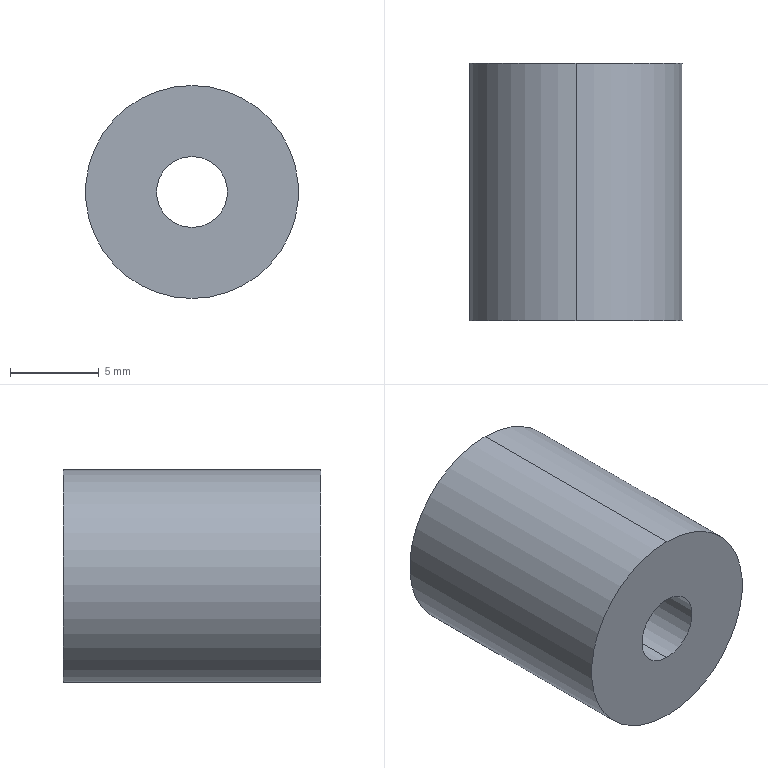Part | STEP file | polyurethane anti-collision post | 1 solid | 9 faces | box 12 x 14.5 x 12 mm | volume 1232 mm3 | cylinder 6 | plane 3 | commonest cylinder face diameters 4 x2 8 x2 12 x2
STEP:
#1=CARTESIAN_POINT('',(0.,0.,0.));
#2=DIRECTION('',(0.,0.,1.));
#3=DIRECTION('',(1.,0.,0.));
#4=AXIS2_PLACEMENT_3D('',#1,#2,#3);
#5=CARTESIAN_POINT('',(0.,8.5,4.));
#6=VERTEX_POINT('',#5);
#7=CARTESIAN_POINT('',(0.,14.5,4.));
#8=VERTEX_POINT('',#7);
#9=CARTESIAN_POINT('',(0.,14.5,4.));
#10=DIRECTION('',(0.,1.,0.));
#11=VECTOR('',#10,1.);
#12=LINE('',#9,#11);
#13=CARTESIAN_POINT('',(0.,14.5,0.));
#14=DIRECTION('',(0.,1.,0.));
#15=DIRECTION('',(0.,0.,1.));
#16=AXIS2_PLACEMENT_3D('',#13,#14,#15);
#17=CYLINDRICAL_SURFACE('',#16,4.);
#18=CARTESIAN_POINT('',(6.283,0.));
#19=DIRECTION('',(0.,1.));
#20=VECTOR('',#19,1.);
#21=LINE('',#18,#20);
#22=(GEOMETRIC_REPRESENTATION_CONTEXT(2)PARAMETRIC_REPRESENTATION_CONTEXT()REPRESENTATION_CONTEXT('',''));
#23=DEFINITIONAL_REPRESENTATION('',(#21),#22);
#24=PCURVE('',#17,#23);
#25=CARTESIAN_POINT('',(0.,14.5,0.));
#26=DIRECTION('',(0.,1.,0.));
#27=DIRECTION('',(0.,0.,1.));
#28=AXIS2_PLACEMENT_3D('',#25,#26,#27);
#29=CYLINDRICAL_SURFACE('',#28,4.);
#30=CARTESIAN_POINT('',(0.,0.));
#31=DIRECTION('',(0.,1.));
#32=VECTOR('',#31,1.);
#33=LINE('',#30,#32);
#34=(GEOMETRIC_REPRESENTATION_CONTEXT(2)PARAMETRIC_REPRESENTATION_CONTEXT()REPRESENTATION_CONTEXT('',''));
#35=DEFINITIONAL_REPRESENTATION('',(#33),#34);
#36=PCURVE('',#29,#35);
#37=SURFACE_CURVE('',#12,(#24,#36),.PCURVE_S1.);
#38=EDGE_CURVE('',#6,#8,#37,.T.);
#39=ORIENTED_EDGE('',*,*,#38,.T.);
#40=CARTESIAN_POINT('',(0.,14.5,-4.));
#41=VERTEX_POINT('',#40);
#42=CARTESIAN_POINT('',(0.,14.5,0.));
#43=DIRECTION('',(0.,1.,0.));
#44=DIRECTION('',(0.,0.,1.));
#45=AXIS2_PLACEMENT_3D('',#42,#43,#44);
#46=CIRCLE('',#45,4.);
#47=CARTESIAN_POINT('',(0.,0.));
#48=DIRECTION('',(1.,0.));
#49=VECTOR('',#48,1.);
#50=LINE('',#47,#49);
#51=(GEOMETRIC_REPRESENTATION_CONTEXT(2)PARAMETRIC_REPRESENTATION_CONTEXT()REPRESENTATION_CONTEXT('',''));
#52=DEFINITIONAL_REPRESENTATION('',(#50),#51);
#53=PCURVE('',#17,#52);
#54=CARTESIAN_POINT('',(0.,14.5,0.));
#55=DIRECTION('',(0.,1.,0.));
#56=DIRECTION('',(0.,0.,1.));
#57=AXIS2_PLACEMENT_3D('',#54,#55,#56);
#58=PLANE('',#57);
#59=CARTESIAN_POINT('',(0.,0.));
#60=DIRECTION('',(1.,0.));
#61=AXIS2_PLACEMENT_2D('',#59,#60);
#62=CIRCLE('',#61,4.);
#63=(GEOMETRIC_REPRESENTATION_CONTEXT(2)PARAMETRIC_REPRESENTATION_CONTEXT()REPRESENTATION_CONTEXT('',''));
#64=DEFINITIONAL_REPRESENTATION('',(#62),#63);
#65=PCURVE('',#58,#64);
#66=SURFACE_CURVE('',#46,(#53,#65),.PCURVE_S1.);
#67=EDGE_CURVE('',#41,#8,#66,.T.);
#68=ORIENTED_EDGE('',*,*,#67,.F.);
#69=CARTESIAN_POINT('',(0.,8.5,-4.));
#70=VERTEX_POINT('',#69);
#71=CARTESIAN_POINT('',(0.,14.5,-4.));
#72=DIRECTION('',(0.,1.,0.));
#73=VECTOR('',#72,1.);
#74=LINE('',#71,#73);
#75=CARTESIAN_POINT('',(3.142,0.));
#76=DIRECTION('',(0.,1.));
#77=VECTOR('',#76,1.);
#78=LINE('',#75,#77);
#79=(GEOMETRIC_REPRESENTATION_CONTEXT(2)PARAMETRIC_REPRESENTATION_CONTEXT()REPRESENTATION_CONTEXT('',''));
#80=DEFINITIONAL_REPRESENTATION('',(#78),#79);
#81=PCURVE('',#17,#80);
#82=CARTESIAN_POINT('',(3.142,0.));
#83=DIRECTION('',(0.,1.));
#84=VECTOR('',#83,1.);
#85=LINE('',#82,#84);
#86=(GEOMETRIC_REPRESENTATION_CONTEXT(2)PARAMETRIC_REPRESENTATION_CONTEXT()REPRESENTATION_CONTEXT('',''));
#87=DEFINITIONAL_REPRESENTATION('',(#85),#86);
#88=PCURVE('',#29,#87);
#89=SURFACE_CURVE('',#74,(#81,#88),.PCURVE_S1.);
#90=EDGE_CURVE('',#70,#41,#89,.T.);
#91=ORIENTED_EDGE('',*,*,#90,.F.);
#92=CARTESIAN_POINT('',(0.,8.5,0.));
#93=DIRECTION('',(0.,1.,0.));
#94=DIRECTION('',(0.,0.,1.));
#95=AXIS2_PLACEMENT_3D('',#92,#93,#94);
#96=CIRCLE('',#95,4.);
#97=CARTESIAN_POINT('',(0.,-6.));
#98=DIRECTION('',(1.,0.));
#99=VECTOR('',#98,1.);
#100=LINE('',#97,#99);
#101=(GEOMETRIC_REPRESENTATION_CONTEXT(2)PARAMETRIC_REPRESENTATION_CONTEXT()REPRESENTATION_CONTEXT('',''));
#102=DEFINITIONAL_REPRESENTATION('',(#100),#101);
#103=PCURVE('',#17,#102);
#104=CARTESIAN_POINT('',(2.,8.5,0.));
#105=DIRECTION('',(0.,-1.,0.));
#106=DIRECTION('',(0.,0.,-1.));
#107=AXIS2_PLACEMENT_3D('',#104,#105,#106);
#108=PLANE('',#107);
#109=CARTESIAN_POINT('',(-4.,-2.));
#110=CARTESIAN_POINT('',(-4.,4.928));
#111=CARTESIAN_POINT('',(2.,1.464));
#112=CARTESIAN_POINT('',(8.,-2.));
#113=CARTESIAN_POINT('',(2.,-5.464));
#114=CARTESIAN_POINT('',(-4.,-8.928));
#115=CARTESIAN_POINT('',(-4.,-2.));
#116=(BOUNDED_CURVE()B_SPLINE_CURVE(2,(#109,#110,#111,#112,#113,#114,#115),.UNSPECIFIED.,.T.,.F.)B_SPLINE_CURVE_WITH_KNOTS((1,2,2,2,2,1),(-2.094,0.,2.094,4.189,6.283,8.378),.UNSPECIFIED.)CURVE()GEOMETRIC_REPRESENTATION_ITEM()RATIONAL_B_SPLINE_CURVE((1.,0.5,1.,0.5,1.,0.5,1.))REPRESENTATION_ITEM(''));
#117=(GEOMETRIC_REPRESENTATION_CONTEXT(2)PARAMETRIC_REPRESENTATION_CONTEXT()REPRESENTATION_CONTEXT('',''));
#118=DEFINITIONAL_REPRESENTATION('',(#116),#117);
#119=PCURVE('',#108,#118);
#120=SURFACE_CURVE('',#96,(#103,#119),.PCURVE_S1.);
#121=EDGE_CURVE('',#70,#6,#120,.T.);
#122=ORIENTED_EDGE('',*,*,#121,.T.);
#123=EDGE_LOOP('',(#39,#68,#91,#122));
#124=FACE_BOUND('',#123,.F.);
#125=ADVANCED_FACE('',(#124),#17,.F.);
#126=CARTESIAN_POINT('',(0.,0.,2.));
#127=VERTEX_POINT('',#126);
#128=CARTESIAN_POINT('',(0.,8.5,2.));
#129=VERTEX_POINT('',#128);
#130=CARTESIAN_POINT('',(0.,14.5,2.));
#131=DIRECTION('',(0.,1.,0.));
#132=VECTOR('',#131,1.);
#133=LINE('',#130,#132);
#134=CARTESIAN_POINT('',(0.,14.5,0.));
#135=DIRECTION('',(0.,1.,0.));
#136=DIRECTION('',(0.,0.,1.));
#137=AXIS2_PLACEMENT_3D('',#134,#135,#136);
#138=CYLINDRICAL_SURFACE('',#137,2.);
#139=CARTESIAN_POINT('',(6.283,0.));
#140=DIRECTION('',(0.,1.));
#141=VECTOR('',#140,1.);
#142=LINE('',#139,#141);
#143=(GEOMETRIC_REPRESENTATION_CONTEXT(2)PARAMETRIC_REPRESENTATION_CONTEXT()REPRESENTATION_CONTEXT('',''));
#144=DEFINITIONAL_REPRESENTATION('',(#142),#143);
#145=PCURVE('',#138,#144);
#146=CARTESIAN_POINT('',(0.,14.5,0.));
#147=DIRECTION('',(0.,1.,0.));
#148=DIRECTION('',(0.,0.,1.));
#149=AXIS2_PLACEMENT_3D('',#146,#147,#148);
#150=CYLINDRICAL_SURFACE('',#149,2.);
#151=CARTESIAN_POINT('',(0.,0.));
#152=DIRECTION('',(0.,1.));
#153=VECTOR('',#152,1.);
#154=LINE('',#151,#153);
#155=(GEOMETRIC_REPRESENTATION_CONTEXT(2)PARAMETRIC_REPRESENTATION_CONTEXT()REPRESENTATION_CONTEXT('',''));
#156=DEFINITIONAL_REPRESENTATION('',(#154),#155);
#157=PCURVE('',#150,#156);
#158=SURFACE_CURVE('',#133,(#145,#157),.PCURVE_S1.);
#159=EDGE_CURVE('',#127,#129,#158,.T.);
#160=ORIENTED_EDGE('',*,*,#159,.T.);
#161=CARTESIAN_POINT('',(0.,8.5,-2.));
#162=VERTEX_POINT('',#161);
#163=CARTESIAN_POINT('',(0.,8.5,0.));
#164=DIRECTION('',(0.,1.,0.));
#165=DIRECTION('',(0.,0.,1.));
#166=AXIS2_PLACEMENT_3D('',#163,#164,#165);
#167=CIRCLE('',#166,2.);
#168=CARTESIAN_POINT('',(0.,-6.));
#169=DIRECTION('',(1.,0.));
#170=VECTOR('',#169,1.);
#171=LINE('',#168,#170);
#172=(GEOMETRIC_REPRESENTATION_CONTEXT(2)PARAMETRIC_REPRESENTATION_CONTEXT()REPRESENTATION_CONTEXT('',''));
#173=DEFINITIONAL_REPRESENTATION('',(#171),#172);
#174=PCURVE('',#138,#173);
#175=CARTESIAN_POINT('',(-2.,-2.));
#176=CARTESIAN_POINT('',(-2.,1.464));
#177=CARTESIAN_POINT('',(1.,-0.2679));
#178=CARTESIAN_POINT('',(4.,-2.));
#179=CARTESIAN_POINT('',(1.,-3.732));
#180=CARTESIAN_POINT('',(-2.,-5.464));
#181=CARTESIAN_POINT('',(-2.,-2.));
#182=(BOUNDED_CURVE()B_SPLINE_CURVE(2,(#175,#176,#177,#178,#179,#180,#181),.UNSPECIFIED.,.T.,.F.)B_SPLINE_CURVE_WITH_KNOTS((1,2,2,2,2,1),(-2.094,0.,2.094,4.189,6.283,8.378),.UNSPECIFIED.)CURVE()GEOMETRIC_REPRESENTATION_ITEM()RATIONAL_B_SPLINE_CURVE((1.,0.5,1.,0.5,1.,0.5,1.))REPRESENTATION_ITEM(''));
#183=(GEOMETRIC_REPRESENTATION_CONTEXT(2)PARAMETRIC_REPRESENTATION_CONTEXT()REPRESENTATION_CONTEXT('',''));
#184=DEFINITIONAL_REPRESENTATION('',(#182),#183);
#185=PCURVE('',#108,#184);
#186=SURFACE_CURVE('',#167,(#174,#185),.PCURVE_S1.);
#187=EDGE_CURVE('',#162,#129,#186,.T.);
#188=ORIENTED_EDGE('',*,*,#187,.F.);
#189=CARTESIAN_POINT('',(0.,0.,-2.));
#190=VERTEX_POINT('',#189);
#191=CARTESIAN_POINT('',(0.,14.5,-2.));
#192=DIRECTION('',(0.,1.,0.));
#193=VECTOR('',#192,1.);
#194=LINE('',#191,#193);
#195=CARTESIAN_POINT('',(3.142,0.));
#196=DIRECTION('',(0.,1.));
#197=VECTOR('',#196,1.);
#198=LINE('',#195,#197);
#199=(GEOMETRIC_REPRESENTATION_CONTEXT(2)PARAMETRIC_REPRESENTATION_CONTEXT()REPRESENTATION_CONTEXT('',''));
#200=DEFINITIONAL_REPRESENTATION('',(#198),#199);
#201=PCURVE('',#138,#200);
#202=CARTESIAN_POINT('',(3.142,0.));
#203=DIRECTION('',(0.,1.));
#204=VECTOR('',#203,1.);
#205=LINE('',#202,#204);
#206=(GEOMETRIC_REPRESENTATION_CONTEXT(2)PARAMETRIC_REPRESENTATION_CONTEXT()REPRESENTATION_CONTEXT('',''));
#207=DEFINITIONAL_REPRESENTATION('',(#205),#206);
#208=PCURVE('',#150,#207);
#209=SURFACE_CURVE('',#194,(#201,#208),.PCURVE_S1.);
#210=EDGE_CURVE('',#190,#162,#209,.T.);
#211=ORIENTED_EDGE('',*,*,#210,.F.);
#212=CARTESIAN_POINT('',(0.,0.,0.));
#213=DIRECTION('',(0.,1.,0.));
#214=DIRECTION('',(0.,0.,1.));
#215=AXIS2_PLACEMENT_3D('',#212,#213,#214);
#216=CIRCLE('',#215,2.);
#217=CARTESIAN_POINT('',(0.,-14.5));
#218=DIRECTION('',(1.,0.));
#219=VECTOR('',#218,1.);
#220=LINE('',#217,#219);
#221=(GEOMETRIC_REPRESENTATION_CONTEXT(2)PARAMETRIC_REPRESENTATION_CONTEXT()REPRESENTATION_CONTEXT('',''));
#222=DEFINITIONAL_REPRESENTATION('',(#220),#221);
#223=PCURVE('',#138,#222);
#224=CARTESIAN_POINT('',(0.,0.,0.));
#225=DIRECTION('',(0.,1.,0.));
#226=DIRECTION('',(0.,0.,1.));
#227=AXIS2_PLACEMENT_3D('',#224,#225,#226);
#228=PLANE('',#227);
#229=CARTESIAN_POINT('',(0.,0.));
#230=DIRECTION('',(1.,0.));
#231=AXIS2_PLACEMENT_2D('',#229,#230);
#232=CIRCLE('',#231,2.);
#233=(GEOMETRIC_REPRESENTATION_CONTEXT(2)PARAMETRIC_REPRESENTATION_CONTEXT()REPRESENTATION_CONTEXT('',''));
#234=DEFINITIONAL_REPRESENTATION('',(#232),#233);
#235=PCURVE('',#228,#234);
#236=SURFACE_CURVE('',#216,(#223,#235),.PCURVE_S1.);
#237=EDGE_CURVE('',#190,#127,#236,.T.);
#238=ORIENTED_EDGE('',*,*,#237,.T.);
#239=EDGE_LOOP('',(#160,#188,#211,#238));
#240=FACE_BOUND('',#239,.F.);
#241=ADVANCED_FACE('',(#240),#138,.F.);
#242=CARTESIAN_POINT('',(0.,14.5,6.));
#243=VERTEX_POINT('',#242);
#244=CARTESIAN_POINT('',(0.,14.5,-6.));
#245=VERTEX_POINT('',#244);
#246=CARTESIAN_POINT('',(0.,14.5,0.));
#247=DIRECTION('',(0.,1.,0.));
#248=DIRECTION('',(0.,0.,1.));
#249=AXIS2_PLACEMENT_3D('',#246,#247,#248);
#250=CIRCLE('',#249,6.);
#251=CARTESIAN_POINT('',(0.,14.5,0.));
#252=DIRECTION('',(0.,-1.,0.));
#253=DIRECTION('',(0.,0.,-1.));
#254=AXIS2_PLACEMENT_3D('',#251,#252,#253);
#255=CYLINDRICAL_SURFACE('',#254,6.);
#256=CARTESIAN_POINT('',(3.142,0.));
#257=DIRECTION('',(-1.,0.));
#258=VECTOR('',#257,1.);
#259=LINE('',#256,#258);
#260=(GEOMETRIC_REPRESENTATION_CONTEXT(2)PARAMETRIC_REPRESENTATION_CONTEXT()REPRESENTATION_CONTEXT('',''));
#261=DEFINITIONAL_REPRESENTATION('',(#259),#260);
#262=PCURVE('',#255,#261);
#263=CARTESIAN_POINT('',(0.,0.));
#264=DIRECTION('',(1.,0.));
#265=AXIS2_PLACEMENT_2D('',#263,#264);
#266=CIRCLE('',#265,6.);
#267=(GEOMETRIC_REPRESENTATION_CONTEXT(2)PARAMETRIC_REPRESENTATION_CONTEXT()REPRESENTATION_CONTEXT('',''));
#268=DEFINITIONAL_REPRESENTATION('',(#266),#267);
#269=PCURVE('',#58,#268);
#270=SURFACE_CURVE('',#250,(#262,#269),.PCURVE_S1.);
#271=EDGE_CURVE('',#243,#245,#270,.T.);
#272=ORIENTED_EDGE('',*,*,#271,.F.);
#273=CARTESIAN_POINT('',(0.,0.,6.));
#274=VERTEX_POINT('',#273);
#275=CARTESIAN_POINT('',(0.,14.5,6.));
#276=DIRECTION('',(0.,-1.,0.));
#277=VECTOR('',#276,1.);
#278=LINE('',#275,#277);
#279=CARTESIAN_POINT('',(3.142,0.));
#280=DIRECTION('',(0.,1.));
#281=VECTOR('',#280,1.);
#282=LINE('',#279,#281);
#283=(GEOMETRIC_REPRESENTATION_CONTEXT(2)PARAMETRIC_REPRESENTATION_CONTEXT()REPRESENTATION_CONTEXT('',''));
#284=DEFINITIONAL_REPRESENTATION('',(#282),#283);
#285=PCURVE('',#255,#284);
#286=CARTESIAN_POINT('',(0.,14.5,0.));
#287=DIRECTION('',(0.,-1.,0.));
#288=DIRECTION('',(0.,0.,-1.));
#289=AXIS2_PLACEMENT_3D('',#286,#287,#288);
#290=CYLINDRICAL_SURFACE('',#289,6.);
#291=CARTESIAN_POINT('',(3.142,0.));
#292=DIRECTION('',(0.,1.));
#293=VECTOR('',#292,1.);
#294=LINE('',#291,#293);
#295=(GEOMETRIC_REPRESENTATION_CONTEXT(2)PARAMETRIC_REPRESENTATION_CONTEXT()REPRESENTATION_CONTEXT('',''));
#296=DEFINITIONAL_REPRESENTATION('',(#294),#295);
#297=PCURVE('',#290,#296);
#298=SURFACE_CURVE('',#278,(#285,#297),.PCURVE_S1.);
#299=EDGE_CURVE('',#243,#274,#298,.T.);
#300=ORIENTED_EDGE('',*,*,#299,.T.);
#301=CARTESIAN_POINT('',(0.,0.,-6.));
#302=VERTEX_POINT('',#301);
#303=CARTESIAN_POINT('',(0.,0.,0.));
#304=DIRECTION('',(0.,1.,0.));
#305=DIRECTION('',(0.,0.,1.));
#306=AXIS2_PLACEMENT_3D('',#303,#304,#305);
#307=CIRCLE('',#306,6.);
#308=CARTESIAN_POINT('',(3.142,14.5));
#309=DIRECTION('',(-1.,0.));
#310=VECTOR('',#309,1.);
#311=LINE('',#308,#310);
#312=(GEOMETRIC_REPRESENTATION_CONTEXT(2)PARAMETRIC_REPRESENTATION_CONTEXT()REPRESENTATION_CONTEXT('',''));
#313=DEFINITIONAL_REPRESENTATION('',(#311),#312);
#314=PCURVE('',#255,#313);
#315=CARTESIAN_POINT('',(0.,0.));
#316=DIRECTION('',(1.,0.));
#317=AXIS2_PLACEMENT_2D('',#315,#316);
#318=CIRCLE('',#317,6.);
#319=(GEOMETRIC_REPRESENTATION_CONTEXT(2)PARAMETRIC_REPRESENTATION_CONTEXT()REPRESENTATION_CONTEXT('',''));
#320=DEFINITIONAL_REPRESENTATION('',(#318),#319);
#321=PCURVE('',#228,#320);
#322=SURFACE_CURVE('',#307,(#314,#321),.PCURVE_S1.);
#323=EDGE_CURVE('',#274,#302,#322,.T.);
#324=ORIENTED_EDGE('',*,*,#323,.T.);
#325=CARTESIAN_POINT('',(0.,14.5,-6.));
#326=DIRECTION('',(0.,-1.,0.));
#327=VECTOR('',#326,1.);
#328=LINE('',#325,#327);
#329=CARTESIAN_POINT('',(0.,0.));
#330=DIRECTION('',(0.,1.));
#331=VECTOR('',#330,1.);
#332=LINE('',#329,#331);
#333=(GEOMETRIC_REPRESENTATION_CONTEXT(2)PARAMETRIC_REPRESENTATION_CONTEXT()REPRESENTATION_CONTEXT('',''));
#334=DEFINITIONAL_REPRESENTATION('',(#332),#333);
#335=PCURVE('',#255,#334);
#336=CARTESIAN_POINT('',(6.283,0.));
#337=DIRECTION('',(0.,1.));
#338=VECTOR('',#337,1.);
#339=LINE('',#336,#338);
#340=(GEOMETRIC_REPRESENTATION_CONTEXT(2)PARAMETRIC_REPRESENTATION_CONTEXT()REPRESENTATION_CONTEXT('',''));
#341=DEFINITIONAL_REPRESENTATION('',(#339),#340);
#342=PCURVE('',#290,#341);
#343=SURFACE_CURVE('',#328,(#335,#342),.PCURVE_S1.);
#344=EDGE_CURVE('',#245,#302,#343,.T.);
#345=ORIENTED_EDGE('',*,*,#344,.F.);
#346=EDGE_LOOP('',(#272,#300,#324,#345));
#347=FACE_BOUND('',#346,.T.);
#348=ADVANCED_FACE('',(#347),#255,.T.);
#349=ORIENTED_EDGE('',*,*,#299,.F.);
#350=CARTESIAN_POINT('',(0.,14.5,0.));
#351=DIRECTION('',(0.,1.,0.));
#352=DIRECTION('',(0.,0.,1.));
#353=AXIS2_PLACEMENT_3D('',#350,#351,#352);
#354=CIRCLE('',#353,6.);
#355=CARTESIAN_POINT('',(9.425,0.));
#356=DIRECTION('',(-1.,0.));
#357=VECTOR('',#356,1.);
#358=LINE('',#355,#357);
#359=(GEOMETRIC_REPRESENTATION_CONTEXT(2)PARAMETRIC_REPRESENTATION_CONTEXT()REPRESENTATION_CONTEXT('',''));
#360=DEFINITIONAL_REPRESENTATION('',(#358),#359);
#361=PCURVE('',#290,#360);
#362=CARTESIAN_POINT('',(0.,0.));
#363=DIRECTION('',(1.,0.));
#364=AXIS2_PLACEMENT_2D('',#362,#363);
#365=CIRCLE('',#364,6.);
#366=(GEOMETRIC_REPRESENTATION_CONTEXT(2)PARAMETRIC_REPRESENTATION_CONTEXT()REPRESENTATION_CONTEXT('',''));
#367=DEFINITIONAL_REPRESENTATION('',(#365),#366);
#368=PCURVE('',#58,#367);
#369=SURFACE_CURVE('',#354,(#361,#368),.PCURVE_S1.);
#370=EDGE_CURVE('',#245,#243,#369,.T.);
#371=ORIENTED_EDGE('',*,*,#370,.F.);
#372=ORIENTED_EDGE('',*,*,#344,.T.);
#373=CARTESIAN_POINT('',(0.,0.,0.));
#374=DIRECTION('',(0.,1.,0.));
#375=DIRECTION('',(0.,0.,1.));
#376=AXIS2_PLACEMENT_3D('',#373,#374,#375);
#377=CIRCLE('',#376,6.);
#378=CARTESIAN_POINT('',(9.425,14.5));
#379=DIRECTION('',(-1.,0.));
#380=VECTOR('',#379,1.);
#381=LINE('',#378,#380);
#382=(GEOMETRIC_REPRESENTATION_CONTEXT(2)PARAMETRIC_REPRESENTATION_CONTEXT()REPRESENTATION_CONTEXT('',''));
#383=DEFINITIONAL_REPRESENTATION('',(#381),#382);
#384=PCURVE('',#290,#383);
#385=CARTESIAN_POINT('',(0.,0.));
#386=DIRECTION('',(1.,0.));
#387=AXIS2_PLACEMENT_2D('',#385,#386);
#388=CIRCLE('',#387,6.);
#389=(GEOMETRIC_REPRESENTATION_CONTEXT(2)PARAMETRIC_REPRESENTATION_CONTEXT()REPRESENTATION_CONTEXT('',''));
#390=DEFINITIONAL_REPRESENTATION('',(#388),#389);
#391=PCURVE('',#228,#390);
#392=SURFACE_CURVE('',#377,(#384,#391),.PCURVE_S1.);
#393=EDGE_CURVE('',#302,#274,#392,.T.);
#394=ORIENTED_EDGE('',*,*,#393,.T.);
#395=EDGE_LOOP('',(#349,#371,#372,#394));
#396=FACE_BOUND('',#395,.T.);
#397=ADVANCED_FACE('',(#396),#290,.T.);
#398=CARTESIAN_POINT('',(0.,14.5,0.));
#399=DIRECTION('',(0.,1.,0.));
#400=DIRECTION('',(0.,0.,1.));
#401=AXIS2_PLACEMENT_3D('',#398,#399,#400);
#402=CIRCLE('',#401,4.);
#403=CARTESIAN_POINT('',(0.,0.));
#404=DIRECTION('',(1.,0.));
#405=AXIS2_PLACEMENT_2D('',#403,#404);
#406=CIRCLE('',#405,4.);
#407=(GEOMETRIC_REPRESENTATION_CONTEXT(2)PARAMETRIC_REPRESENTATION_CONTEXT()REPRESENTATION_CONTEXT('',''));
#408=DEFINITIONAL_REPRESENTATION('',(#406),#407);
#409=PCURVE('',#58,#408);
#410=CARTESIAN_POINT('',(0.,0.));
#411=DIRECTION('',(1.,0.));
#412=VECTOR('',#411,1.);
#413=LINE('',#410,#412);
#414=(GEOMETRIC_REPRESENTATION_CONTEXT(2)PARAMETRIC_REPRESENTATION_CONTEXT()REPRESENTATION_CONTEXT('',''));
#415=DEFINITIONAL_REPRESENTATION('',(#413),#414);
#416=PCURVE('',#29,#415);
#417=SURFACE_CURVE('',#402,(#409,#416),.PCURVE_S1.);
#418=EDGE_CURVE('',#8,#41,#417,.T.);
#419=ORIENTED_EDGE('',*,*,#418,.F.);
#420=ORIENTED_EDGE('',*,*,#67,.F.);
#421=EDGE_LOOP('',(#419,#420));
#422=FACE_BOUND('',#421,.T.);
#423=ORIENTED_EDGE('',*,*,#370,.T.);
#424=ORIENTED_EDGE('',*,*,#271,.T.);
#425=EDGE_LOOP('',(#423,#424));
#426=FACE_BOUND('',#425,.T.);
#427=ADVANCED_FACE('',(#422,#426),#58,.T.);
#428=CARTESIAN_POINT('',(0.,0.,0.));
#429=DIRECTION('',(0.,1.,0.));
#430=DIRECTION('',(0.,0.,1.));
#431=AXIS2_PLACEMENT_3D('',#428,#429,#430);
#432=CIRCLE('',#431,2.);
#433=CARTESIAN_POINT('',(0.,0.));
#434=DIRECTION('',(1.,0.));
#435=AXIS2_PLACEMENT_2D('',#433,#434);
#436=CIRCLE('',#435,2.);
#437=(GEOMETRIC_REPRESENTATION_CONTEXT(2)PARAMETRIC_REPRESENTATION_CONTEXT()REPRESENTATION_CONTEXT('',''));
#438=DEFINITIONAL_REPRESENTATION('',(#436),#437);
#439=PCURVE('',#228,#438);
#440=CARTESIAN_POINT('',(0.,-14.5));
#441=DIRECTION('',(1.,0.));
#442=VECTOR('',#441,1.);
#443=LINE('',#440,#442);
#444=(GEOMETRIC_REPRESENTATION_CONTEXT(2)PARAMETRIC_REPRESENTATION_CONTEXT()REPRESENTATION_CONTEXT('',''));
#445=DEFINITIONAL_REPRESENTATION('',(#443),#444);
#446=PCURVE('',#150,#445);
#447=SURFACE_CURVE('',#432,(#439,#446),.PCURVE_S1.);
#448=EDGE_CURVE('',#127,#190,#447,.T.);
#449=ORIENTED_EDGE('',*,*,#448,.T.);
#450=ORIENTED_EDGE('',*,*,#237,.T.);
#451=EDGE_LOOP('',(#449,#450));
#452=FACE_BOUND('',#451,.T.);
#453=ORIENTED_EDGE('',*,*,#393,.F.);
#454=ORIENTED_EDGE('',*,*,#323,.F.);
#455=EDGE_LOOP('',(#453,#454));
#456=FACE_BOUND('',#455,.T.);
#457=ADVANCED_FACE('',(#452,#456),#228,.F.);
#458=CARTESIAN_POINT('',(0.,8.5,0.));
#459=DIRECTION('',(0.,1.,0.));
#460=DIRECTION('',(0.,0.,1.));
#461=AXIS2_PLACEMENT_3D('',#458,#459,#460);
#462=CIRCLE('',#461,2.);
#463=CARTESIAN_POINT('',(0.,-6.));
#464=DIRECTION('',(1.,0.));
#465=VECTOR('',#464,1.);
#466=LINE('',#463,#465);
#467=(GEOMETRIC_REPRESENTATION_CONTEXT(2)PARAMETRIC_REPRESENTATION_CONTEXT()REPRESENTATION_CONTEXT('',''));
#468=DEFINITIONAL_REPRESENTATION('',(#466),#467);
#469=PCURVE('',#150,#468);
#470=CARTESIAN_POINT('',(-2.,-2.));
#471=CARTESIAN_POINT('',(-2.,1.464));
#472=CARTESIAN_POINT('',(1.,-0.2679));
#473=CARTESIAN_POINT('',(4.,-2.));
#474=CARTESIAN_POINT('',(1.,-3.732));
#475=CARTESIAN_POINT('',(-2.,-5.464));
#476=CARTESIAN_POINT('',(-2.,-2.));
#477=(BOUNDED_CURVE()B_SPLINE_CURVE(2,(#470,#471,#472,#473,#474,#475,#476),.UNSPECIFIED.,.T.,.F.)B_SPLINE_CURVE_WITH_KNOTS((1,2,2,2,2,1),(-2.094,0.,2.094,4.189,6.283,8.378),.UNSPECIFIED.)CURVE()GEOMETRIC_REPRESENTATION_ITEM()RATIONAL_B_SPLINE_CURVE((1.,0.5,1.,0.5,1.,0.5,1.))REPRESENTATION_ITEM(''));
#478=(GEOMETRIC_REPRESENTATION_CONTEXT(2)PARAMETRIC_REPRESENTATION_CONTEXT()REPRESENTATION_CONTEXT('',''));
#479=DEFINITIONAL_REPRESENTATION('',(#477),#478);
#480=PCURVE('',#108,#479);
#481=SURFACE_CURVE('',#462,(#469,#480),.PCURVE_S1.);
#482=EDGE_CURVE('',#129,#162,#481,.T.);
#483=ORIENTED_EDGE('',*,*,#482,.F.);
#484=ORIENTED_EDGE('',*,*,#159,.F.);
#485=ORIENTED_EDGE('',*,*,#448,.T.);
#486=ORIENTED_EDGE('',*,*,#210,.T.);
#487=EDGE_LOOP('',(#483,#484,#485,#486));
#488=FACE_BOUND('',#487,.F.);
#489=ADVANCED_FACE('',(#488),#150,.F.);
#490=ORIENTED_EDGE('',*,*,#482,.F.);
#491=ORIENTED_EDGE('',*,*,#187,.F.);
#492=EDGE_LOOP('',(#490,#491));
#493=FACE_BOUND('',#492,.T.);
#494=CARTESIAN_POINT('',(0.,8.5,0.));
#495=DIRECTION('',(0.,1.,0.));
#496=DIRECTION('',(0.,0.,1.));
#497=AXIS2_PLACEMENT_3D('',#494,#495,#496);
#498=CIRCLE('',#497,4.);
#499=CARTESIAN_POINT('',(-4.,-2.));
#500=CARTESIAN_POINT('',(-4.,4.928));
#501=CARTESIAN_POINT('',(2.,1.464));
#502=CARTESIAN_POINT('',(8.,-2.));
#503=CARTESIAN_POINT('',(2.,-5.464));
#504=CARTESIAN_POINT('',(-4.,-8.928));
#505=CARTESIAN_POINT('',(-4.,-2.));
#506=(BOUNDED_CURVE()B_SPLINE_CURVE(2,(#499,#500,#501,#502,#503,#504,#505),.UNSPECIFIED.,.T.,.F.)B_SPLINE_CURVE_WITH_KNOTS((1,2,2,2,2,1),(-2.094,0.,2.094,4.189,6.283,8.378),.UNSPECIFIED.)CURVE()GEOMETRIC_REPRESENTATION_ITEM()RATIONAL_B_SPLINE_CURVE((1.,0.5,1.,0.5,1.,0.5,1.))REPRESENTATION_ITEM(''));
#507=(GEOMETRIC_REPRESENTATION_CONTEXT(2)PARAMETRIC_REPRESENTATION_CONTEXT()REPRESENTATION_CONTEXT('',''));
#508=DEFINITIONAL_REPRESENTATION('',(#506),#507);
#509=PCURVE('',#108,#508);
#510=CARTESIAN_POINT('',(0.,-6.));
#511=DIRECTION('',(1.,0.));
#512=VECTOR('',#511,1.);
#513=LINE('',#510,#512);
#514=(GEOMETRIC_REPRESENTATION_CONTEXT(2)PARAMETRIC_REPRESENTATION_CONTEXT()REPRESENTATION_CONTEXT('',''));
#515=DEFINITIONAL_REPRESENTATION('',(#513),#514);
#516=PCURVE('',#29,#515);
#517=SURFACE_CURVE('',#498,(#509,#516),.PCURVE_S1.);
#518=EDGE_CURVE('',#6,#70,#517,.T.);
#519=ORIENTED_EDGE('',*,*,#518,.T.);
#520=ORIENTED_EDGE('',*,*,#121,.T.);
#521=EDGE_LOOP('',(#519,#520));
#522=FACE_BOUND('',#521,.T.);
#523=ADVANCED_FACE('',(#493,#522),#108,.F.);
#524=ORIENTED_EDGE('',*,*,#418,.F.);
#525=ORIENTED_EDGE('',*,*,#38,.F.);
#526=ORIENTED_EDGE('',*,*,#518,.T.);
#527=ORIENTED_EDGE('',*,*,#90,.T.);
#528=EDGE_LOOP('',(#524,#525,#526,#527));
#529=FACE_BOUND('',#528,.F.);
#530=ADVANCED_FACE('',(#529),#29,.F.);
#531=CLOSED_SHELL('',(#125,#241,#348,#397,#427,#457,#489,#523,#530));
#532=MANIFOLD_SOLID_BREP('',#531);
#533=(LENGTH_UNIT()NAMED_UNIT(*)SI_UNIT(.MILLI.,.METRE.));
#534=UNCERTAINTY_MEASURE_WITH_UNIT(LENGTH_MEASURE(0.0000001),#533,'','');
#535=(NAMED_UNIT(*)PLANE_ANGLE_UNIT()SI_UNIT($,.RADIAN.));
#536=(NAMED_UNIT(*)SI_UNIT($,.STERADIAN.)SOLID_ANGLE_UNIT());
#537=(GEOMETRIC_REPRESENTATION_CONTEXT(3)GLOBAL_UNCERTAINTY_ASSIGNED_CONTEXT((#534))GLOBAL_UNIT_ASSIGNED_CONTEXT((#533,#535,#536))REPRESENTATION_CONTEXT('',''));
#538=ADVANCED_BREP_SHAPE_REPRESENTATION('',(#4,#532),#537);